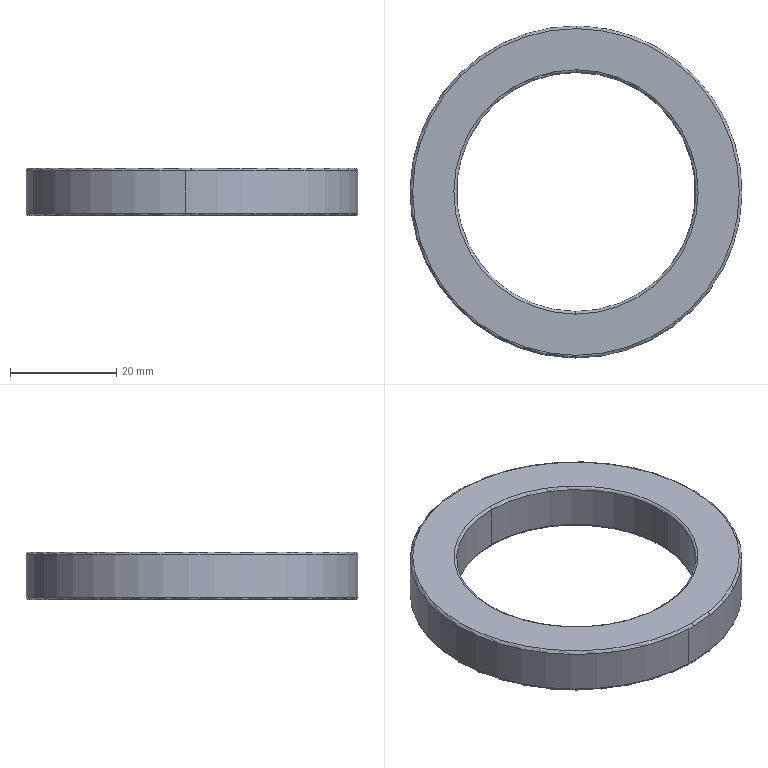Part | STEP file | 2026.6.15-Main Assembly图.sldasm-Part-147 | 1 solid | 14 faces | box 62.5 x 62.5 x 9 mm | volume 13262 mm3 | torus 8 | cylinder 4 | plane 2 | commonest cylinder face diameters 45 x2 62.5 x2
STEP:
#1=CARTESIAN_POINT('',(-1571.277,1393.006,3633.071));
#2=VERTEX_POINT('',#1);
#3=CARTESIAN_POINT('',(-1570.037,1455.482,3633.071));
#4=VERTEX_POINT('',#3);
#5=CARTESIAN_POINT('',(-1571.253,1424.256,3633.071));
#6=DIRECTION('',(0.,0.,1.));
#7=DIRECTION('',(0.0007664,1.,0.));
#8=AXIS2_PLACEMENT_3D('',#5,#6,#7);
#9=CIRCLE('',#8,31.25);
#10=EDGE_CURVE('',#2,#4,#9,.T.);
#11=ORIENTED_EDGE('',*,*,#10,.F.);
#12=CARTESIAN_POINT('',(-1571.277,1393.506,3632.571));
#13=VERTEX_POINT('',#12);
#14=CARTESIAN_POINT('',(-1571.277,1393.506,3633.071));
#15=DIRECTION('',(1.,-0.0007664,0.));
#16=DIRECTION('',(0.0007664,1.,0.));
#17=AXIS2_PLACEMENT_3D('',#14,#15,#16);
#18=CIRCLE('',#17,0.5);
#19=EDGE_CURVE('',#2,#13,#18,.T.);
#20=ORIENTED_EDGE('',*,*,#19,.T.);
#21=CARTESIAN_POINT('',(-1571.23,1455.006,3632.571));
#22=VERTEX_POINT('',#21);
#23=CARTESIAN_POINT('',(-1571.253,1424.256,3632.571));
#24=DIRECTION('',(0.,0.,-1.));
#25=DIRECTION('',(0.0007664,1.,0.));
#26=AXIS2_PLACEMENT_3D('',#23,#24,#25);
#27=CIRCLE('',#26,30.75);
#28=EDGE_CURVE('',#22,#13,#27,.T.);
#29=ORIENTED_EDGE('',*,*,#28,.F.);
#30=CARTESIAN_POINT('',(-1571.229,1455.506,3633.071));
#31=VERTEX_POINT('',#30);
#32=CARTESIAN_POINT('',(-1571.23,1455.006,3633.071));
#33=DIRECTION('',(-1.,0.0007664,0.));
#34=DIRECTION('',(-0.0007664,-1.,0.));
#35=AXIS2_PLACEMENT_3D('',#32,#33,#34);
#36=CIRCLE('',#35,0.5);
#37=EDGE_CURVE('',#31,#22,#36,.T.);
#38=ORIENTED_EDGE('',*,*,#37,.F.);
#39=CARTESIAN_POINT('',(-1571.253,1424.256,3633.071));
#40=DIRECTION('',(0.,0.,1.));
#41=DIRECTION('',(0.0007664,1.,0.));
#42=AXIS2_PLACEMENT_3D('',#39,#40,#41);
#43=CIRCLE('',#42,31.25);
#44=EDGE_CURVE('',#4,#31,#43,.T.);
#45=ORIENTED_EDGE('',*,*,#44,.F.);
#46=EDGE_LOOP('',(#11,#20,#29,#38,#45));
#47=FACE_OUTER_BOUND('',#46,.T.);
#48=CARTESIAN_POINT('',(-1571.253,1424.256,3633.071));
#49=DIRECTION('',(0.,0.,-1.));
#50=DIRECTION('',(0.0007664,1.,0.));
#51=AXIS2_PLACEMENT_3D('',#48,#49,#50);
#52=TOROIDAL_SURFACE('',#51,30.75,0.5);
#53=ADVANCED_FACE('',(#47),#52,.T.);
#54=CARTESIAN_POINT('',(-1571.229,1455.506,3641.071));
#55=VERTEX_POINT('',#54);
#56=CARTESIAN_POINT('',(-1570.037,1455.482,3641.071));
#57=VERTEX_POINT('',#56);
#58=CARTESIAN_POINT('',(-1571.253,1424.256,3641.071));
#59=DIRECTION('',(0.,0.,-1.));
#60=DIRECTION('',(-0.0007664,-1.,0.));
#61=AXIS2_PLACEMENT_3D('',#58,#59,#60);
#62=CIRCLE('',#61,31.25);
#63=EDGE_CURVE('',#55,#57,#62,.T.);
#64=ORIENTED_EDGE('',*,*,#63,.F.);
#65=CARTESIAN_POINT('',(-1571.23,1455.006,3641.571));
#66=VERTEX_POINT('',#65);
#67=CARTESIAN_POINT('',(-1571.23,1455.006,3641.071));
#68=DIRECTION('',(1.,-0.0007664,0.));
#69=DIRECTION('',(0.0007664,1.,0.));
#70=AXIS2_PLACEMENT_3D('',#67,#68,#69);
#71=CIRCLE('',#70,0.5);
#72=EDGE_CURVE('',#55,#66,#71,.T.);
#73=ORIENTED_EDGE('',*,*,#72,.T.);
#74=CARTESIAN_POINT('',(-1571.277,1393.506,3641.571));
#75=VERTEX_POINT('',#74);
#76=CARTESIAN_POINT('',(-1571.253,1424.256,3641.571));
#77=DIRECTION('',(0.,0.,1.));
#78=DIRECTION('',(-0.0007664,-1.,0.));
#79=AXIS2_PLACEMENT_3D('',#76,#77,#78);
#80=CIRCLE('',#79,30.75);
#81=EDGE_CURVE('',#75,#66,#80,.T.);
#82=ORIENTED_EDGE('',*,*,#81,.F.);
#83=CARTESIAN_POINT('',(-1571.277,1393.006,3641.071));
#84=VERTEX_POINT('',#83);
#85=CARTESIAN_POINT('',(-1571.277,1393.506,3641.071));
#86=DIRECTION('',(-1.,0.0007664,0.));
#87=DIRECTION('',(-0.0007664,-1.,0.));
#88=AXIS2_PLACEMENT_3D('',#85,#86,#87);
#89=CIRCLE('',#88,0.5);
#90=EDGE_CURVE('',#84,#75,#89,.T.);
#91=ORIENTED_EDGE('',*,*,#90,.F.);
#92=CARTESIAN_POINT('',(-1571.253,1424.256,3641.071));
#93=DIRECTION('',(0.,0.,-1.));
#94=DIRECTION('',(-0.0007664,-1.,0.));
#95=AXIS2_PLACEMENT_3D('',#92,#93,#94);
#96=CIRCLE('',#95,31.25);
#97=EDGE_CURVE('',#57,#84,#96,.T.);
#98=ORIENTED_EDGE('',*,*,#97,.F.);
#99=EDGE_LOOP('',(#64,#73,#82,#91,#98));
#100=FACE_OUTER_BOUND('',#99,.T.);
#101=CARTESIAN_POINT('',(-1571.253,1424.256,3641.071));
#102=DIRECTION('',(0.,0.,1.));
#103=DIRECTION('',(-0.0007664,-1.,0.));
#104=AXIS2_PLACEMENT_3D('',#101,#102,#103);
#105=TOROIDAL_SURFACE('',#104,30.75,0.5);
#106=ADVANCED_FACE('',(#100),#105,.T.);
#107=CARTESIAN_POINT('',(-1571.236,1447.256,3641.571));
#108=VERTEX_POINT('',#107);
#109=CARTESIAN_POINT('',(-1571.271,1401.256,3641.571));
#110=VERTEX_POINT('',#109);
#111=CARTESIAN_POINT('',(-1571.253,1424.256,3641.571));
#112=DIRECTION('',(0.,0.,-1.));
#113=DIRECTION('',(-0.0007664,-1.,0.));
#114=AXIS2_PLACEMENT_3D('',#111,#112,#113);
#115=CIRCLE('',#114,23.);
#116=EDGE_CURVE('',#108,#110,#115,.T.);
#117=ORIENTED_EDGE('',*,*,#116,.F.);
#118=CARTESIAN_POINT('',(-1571.236,1446.756,3641.071));
#119=VERTEX_POINT('',#118);
#120=CARTESIAN_POINT('',(-1571.236,1447.256,3641.071));
#121=DIRECTION('',(1.,-0.0007664,0.));
#122=DIRECTION('',(0.0007664,1.,0.));
#123=AXIS2_PLACEMENT_3D('',#120,#121,#122);
#124=CIRCLE('',#123,0.5);
#125=EDGE_CURVE('',#108,#119,#124,.T.);
#126=ORIENTED_EDGE('',*,*,#125,.T.);
#127=CARTESIAN_POINT('',(-1571.27,1401.756,3641.071));
#128=VERTEX_POINT('',#127);
#129=CARTESIAN_POINT('',(-1571.253,1424.256,3641.071));
#130=DIRECTION('',(0.,0.,1.));
#131=DIRECTION('',(-0.0007664,-1.,0.));
#132=AXIS2_PLACEMENT_3D('',#129,#130,#131);
#133=CIRCLE('',#132,22.5);
#134=EDGE_CURVE('',#128,#119,#133,.T.);
#135=ORIENTED_EDGE('',*,*,#134,.F.);
#136=CARTESIAN_POINT('',(-1571.271,1401.256,3641.071));
#137=DIRECTION('',(-1.,0.0007664,0.));
#138=DIRECTION('',(-0.0007664,-1.,0.));
#139=AXIS2_PLACEMENT_3D('',#136,#137,#138);
#140=CIRCLE('',#139,0.5);
#141=EDGE_CURVE('',#110,#128,#140,.T.);
#142=ORIENTED_EDGE('',*,*,#141,.F.);
#143=EDGE_LOOP('',(#117,#126,#135,#142));
#144=FACE_OUTER_BOUND('',#143,.T.);
#145=CARTESIAN_POINT('',(-1571.253,1424.256,3641.071));
#146=DIRECTION('',(0.,0.,1.));
#147=DIRECTION('',(-0.0007664,-1.,0.));
#148=AXIS2_PLACEMENT_3D('',#145,#146,#147);
#149=TOROIDAL_SURFACE('',#148,23.,0.5);
#150=ADVANCED_FACE('',(#144),#149,.T.);
#151=CARTESIAN_POINT('',(-1571.271,1401.256,3632.571));
#152=VERTEX_POINT('',#151);
#153=CARTESIAN_POINT('',(-1571.236,1447.256,3632.571));
#154=VERTEX_POINT('',#153);
#155=CARTESIAN_POINT('',(-1571.253,1424.256,3632.571));
#156=DIRECTION('',(0.,0.,1.));
#157=DIRECTION('',(0.0007664,1.,0.));
#158=AXIS2_PLACEMENT_3D('',#155,#156,#157);
#159=CIRCLE('',#158,23.);
#160=EDGE_CURVE('',#152,#154,#159,.T.);
#161=ORIENTED_EDGE('',*,*,#160,.F.);
#162=CARTESIAN_POINT('',(-1571.27,1401.756,3633.071));
#163=VERTEX_POINT('',#162);
#164=CARTESIAN_POINT('',(-1571.271,1401.256,3633.071));
#165=DIRECTION('',(1.,-0.0007664,0.));
#166=DIRECTION('',(0.0007664,1.,0.));
#167=AXIS2_PLACEMENT_3D('',#164,#165,#166);
#168=CIRCLE('',#167,0.5);
#169=EDGE_CURVE('',#152,#163,#168,.T.);
#170=ORIENTED_EDGE('',*,*,#169,.T.);
#171=CARTESIAN_POINT('',(-1571.236,1446.756,3633.071));
#172=VERTEX_POINT('',#171);
#173=CARTESIAN_POINT('',(-1571.253,1424.256,3633.071));
#174=DIRECTION('',(0.,0.,-1.));
#175=DIRECTION('',(0.0007664,1.,0.));
#176=AXIS2_PLACEMENT_3D('',#173,#174,#175);
#177=CIRCLE('',#176,22.5);
#178=EDGE_CURVE('',#172,#163,#177,.T.);
#179=ORIENTED_EDGE('',*,*,#178,.F.);
#180=CARTESIAN_POINT('',(-1571.236,1447.256,3633.071));
#181=DIRECTION('',(-1.,0.0007664,0.));
#182=DIRECTION('',(-0.0007664,-1.,0.));
#183=AXIS2_PLACEMENT_3D('',#180,#181,#182);
#184=CIRCLE('',#183,0.5);
#185=EDGE_CURVE('',#154,#172,#184,.T.);
#186=ORIENTED_EDGE('',*,*,#185,.F.);
#187=EDGE_LOOP('',(#161,#170,#179,#186));
#188=FACE_OUTER_BOUND('',#187,.T.);
#189=CARTESIAN_POINT('',(-1571.253,1424.256,3633.071));
#190=DIRECTION('',(0.,0.,-1.));
#191=DIRECTION('',(0.0007664,1.,0.));
#192=AXIS2_PLACEMENT_3D('',#189,#190,#191);
#193=TOROIDAL_SURFACE('',#192,23.,0.5);
#194=ADVANCED_FACE('',(#188),#193,.T.);
#195=CARTESIAN_POINT('',(-1571.253,1424.256,3633.071));
#196=DIRECTION('',(0.,0.,-1.));
#197=DIRECTION('',(0.0007664,1.,0.));
#198=AXIS2_PLACEMENT_3D('',#195,#196,#197);
#199=CIRCLE('',#198,22.5);
#200=EDGE_CURVE('',#163,#172,#199,.T.);
#201=ORIENTED_EDGE('',*,*,#200,.T.);
#202=CARTESIAN_POINT('',(-1571.236,1446.756,3632.571));
#203=DIRECTION('',(0.,0.,1.));
#204=VECTOR('',#203,1000.);
#205=LINE('',#202,#204);
#206=EDGE_CURVE('',#172,#119,#205,.T.);
#207=ORIENTED_EDGE('',*,*,#206,.T.);
#208=CARTESIAN_POINT('',(-1571.253,1424.256,3641.071));
#209=DIRECTION('',(0.,0.,1.));
#210=DIRECTION('',(-0.0007664,-1.,0.));
#211=AXIS2_PLACEMENT_3D('',#208,#209,#210);
#212=CIRCLE('',#211,22.5);
#213=EDGE_CURVE('',#119,#128,#212,.T.);
#214=ORIENTED_EDGE('',*,*,#213,.T.);
#215=CARTESIAN_POINT('',(-1571.27,1401.756,3632.571));
#216=DIRECTION('',(0.,0.,1.));
#217=VECTOR('',#216,1000.);
#218=LINE('',#215,#217);
#219=EDGE_CURVE('',#163,#128,#218,.T.);
#220=ORIENTED_EDGE('',*,*,#219,.F.);
#221=EDGE_LOOP('',(#201,#207,#214,#220));
#222=FACE_OUTER_BOUND('',#221,.T.);
#223=CARTESIAN_POINT('',(-1571.253,1424.256,3632.571));
#224=DIRECTION('',(0.,0.,1.));
#225=DIRECTION('',(-0.0007664,-1.,0.));
#226=AXIS2_PLACEMENT_3D('',#223,#224,#225);
#227=CYLINDRICAL_SURFACE('',#226,22.5);
#228=ADVANCED_FACE('',(#222),#227,.F.);
#229=ORIENTED_EDGE('',*,*,#97,.T.);
#230=CARTESIAN_POINT('',(-1572.469,1393.03,3641.071));
#231=VERTEX_POINT('',#230);
#232=CARTESIAN_POINT('',(-1571.253,1424.256,3641.071));
#233=DIRECTION('',(0.,0.,-1.));
#234=DIRECTION('',(-0.0007664,-1.,0.));
#235=AXIS2_PLACEMENT_3D('',#232,#233,#234);
#236=CIRCLE('',#235,31.25);
#237=EDGE_CURVE('',#84,#231,#236,.T.);
#238=ORIENTED_EDGE('',*,*,#237,.T.);
#239=CARTESIAN_POINT('',(-1572.469,1393.03,3633.071));
#240=VERTEX_POINT('',#239);
#241=CARTESIAN_POINT('',(-1572.469,1393.03,3641.571));
#242=DIRECTION('',(0.,0.,-1.));
#243=VECTOR('',#242,1000.);
#244=LINE('',#241,#243);
#245=EDGE_CURVE('',#231,#240,#244,.T.);
#246=ORIENTED_EDGE('',*,*,#245,.T.);
#247=CARTESIAN_POINT('',(-1571.253,1424.256,3633.071));
#248=DIRECTION('',(0.,0.,1.));
#249=DIRECTION('',(0.0007664,1.,0.));
#250=AXIS2_PLACEMENT_3D('',#247,#248,#249);
#251=CIRCLE('',#250,31.25);
#252=EDGE_CURVE('',#240,#2,#251,.T.);
#253=ORIENTED_EDGE('',*,*,#252,.T.);
#254=ORIENTED_EDGE('',*,*,#10,.T.);
#255=CARTESIAN_POINT('',(-1570.037,1455.482,3641.571));
#256=DIRECTION('',(0.,0.,-1.));
#257=VECTOR('',#256,1000.);
#258=LINE('',#255,#257);
#259=EDGE_CURVE('',#57,#4,#258,.T.);
#260=ORIENTED_EDGE('',*,*,#259,.F.);
#261=EDGE_LOOP('',(#229,#238,#246,#253,#254,#260));
#262=FACE_OUTER_BOUND('',#261,.T.);
#263=CARTESIAN_POINT('',(-1571.253,1424.256,3641.571));
#264=DIRECTION('',(0.,0.,-1.));
#265=DIRECTION('',(0.03892,0.9992,0.));
#266=AXIS2_PLACEMENT_3D('',#263,#264,#265);
#267=CYLINDRICAL_SURFACE('',#266,31.25);
#268=ADVANCED_FACE('',(#262),#267,.T.);
#269=CARTESIAN_POINT('',(-1571.253,1424.256,3632.571));
#270=DIRECTION('',(0.,0.,1.));
#271=DIRECTION('',(0.0007664,1.,0.));
#272=AXIS2_PLACEMENT_3D('',#269,#270,#271);
#273=CIRCLE('',#272,23.);
#274=EDGE_CURVE('',#154,#152,#273,.T.);
#275=ORIENTED_EDGE('',*,*,#274,.T.);
#276=ORIENTED_EDGE('',*,*,#160,.T.);
#277=EDGE_LOOP('',(#275,#276));
#278=FACE_BOUND('',#277,.T.);
#279=ORIENTED_EDGE('',*,*,#28,.T.);
#280=CARTESIAN_POINT('',(-1571.253,1424.256,3632.571));
#281=DIRECTION('',(0.,0.,-1.));
#282=DIRECTION('',(0.0007664,1.,0.));
#283=AXIS2_PLACEMENT_3D('',#280,#281,#282);
#284=CIRCLE('',#283,30.75);
#285=EDGE_CURVE('',#13,#22,#284,.T.);
#286=ORIENTED_EDGE('',*,*,#285,.T.);
#287=EDGE_LOOP('',(#279,#286));
#288=FACE_OUTER_BOUND('',#287,.T.);
#289=CARTESIAN_POINT('',(-1571.253,1424.256,3632.571));
#290=DIRECTION('',(0.,0.,-1.));
#291=DIRECTION('',(0.0007664,1.,0.));
#292=AXIS2_PLACEMENT_3D('',#289,#290,#291);
#293=PLANE('',#292);
#294=ADVANCED_FACE('',(#278,#288),#293,.T.);
#295=CARTESIAN_POINT('',(-1571.253,1424.256,3641.571));
#296=DIRECTION('',(0.,0.,-1.));
#297=DIRECTION('',(-0.0007664,-1.,0.));
#298=AXIS2_PLACEMENT_3D('',#295,#296,#297);
#299=CIRCLE('',#298,23.);
#300=EDGE_CURVE('',#110,#108,#299,.T.);
#301=ORIENTED_EDGE('',*,*,#300,.T.);
#302=ORIENTED_EDGE('',*,*,#116,.T.);
#303=EDGE_LOOP('',(#301,#302));
#304=FACE_BOUND('',#303,.T.);
#305=ORIENTED_EDGE('',*,*,#81,.T.);
#306=CARTESIAN_POINT('',(-1571.253,1424.256,3641.571));
#307=DIRECTION('',(0.,0.,1.));
#308=DIRECTION('',(-0.0007664,-1.,0.));
#309=AXIS2_PLACEMENT_3D('',#306,#307,#308);
#310=CIRCLE('',#309,30.75);
#311=EDGE_CURVE('',#66,#75,#310,.T.);
#312=ORIENTED_EDGE('',*,*,#311,.T.);
#313=EDGE_LOOP('',(#305,#312));
#314=FACE_OUTER_BOUND('',#313,.T.);
#315=CARTESIAN_POINT('',(-1571.253,1424.256,3641.571));
#316=DIRECTION('',(0.,0.,1.));
#317=DIRECTION('',(-0.0007664,-1.,0.));
#318=AXIS2_PLACEMENT_3D('',#315,#316,#317);
#319=PLANE('',#318);
#320=ADVANCED_FACE('',(#304,#314),#319,.T.);
#321=ORIENTED_EDGE('',*,*,#245,.F.);
#322=CARTESIAN_POINT('',(-1571.253,1424.256,3641.071));
#323=DIRECTION('',(0.,0.,-1.));
#324=DIRECTION('',(-0.0007664,-1.,0.));
#325=AXIS2_PLACEMENT_3D('',#322,#323,#324);
#326=CIRCLE('',#325,31.25);
#327=EDGE_CURVE('',#231,#55,#326,.T.);
#328=ORIENTED_EDGE('',*,*,#327,.T.);
#329=ORIENTED_EDGE('',*,*,#63,.T.);
#330=ORIENTED_EDGE('',*,*,#259,.T.);
#331=ORIENTED_EDGE('',*,*,#44,.T.);
#332=CARTESIAN_POINT('',(-1571.253,1424.256,3633.071));
#333=DIRECTION('',(0.,0.,1.));
#334=DIRECTION('',(0.0007664,1.,0.));
#335=AXIS2_PLACEMENT_3D('',#332,#333,#334);
#336=CIRCLE('',#335,31.25);
#337=EDGE_CURVE('',#31,#240,#336,.T.);
#338=ORIENTED_EDGE('',*,*,#337,.T.);
#339=EDGE_LOOP('',(#321,#328,#329,#330,#331,#338));
#340=FACE_OUTER_BOUND('',#339,.T.);
#341=CARTESIAN_POINT('',(-1571.253,1424.256,3641.571));
#342=DIRECTION('',(0.,0.,-1.));
#343=DIRECTION('',(0.03892,0.9992,0.));
#344=AXIS2_PLACEMENT_3D('',#341,#342,#343);
#345=CYLINDRICAL_SURFACE('',#344,31.25);
#346=ADVANCED_FACE('',(#340),#345,.T.);
#347=ORIENTED_EDGE('',*,*,#206,.F.);
#348=ORIENTED_EDGE('',*,*,#178,.T.);
#349=ORIENTED_EDGE('',*,*,#219,.T.);
#350=ORIENTED_EDGE('',*,*,#134,.T.);
#351=EDGE_LOOP('',(#347,#348,#349,#350));
#352=FACE_OUTER_BOUND('',#351,.T.);
#353=CARTESIAN_POINT('',(-1571.253,1424.256,3632.571));
#354=DIRECTION('',(0.,0.,1.));
#355=DIRECTION('',(-0.0007664,-1.,0.));
#356=AXIS2_PLACEMENT_3D('',#353,#354,#355);
#357=CYLINDRICAL_SURFACE('',#356,22.5);
#358=ADVANCED_FACE('',(#352),#357,.F.);
#359=ORIENTED_EDGE('',*,*,#169,.F.);
#360=ORIENTED_EDGE('',*,*,#274,.F.);
#361=ORIENTED_EDGE('',*,*,#185,.T.);
#362=ORIENTED_EDGE('',*,*,#200,.F.);
#363=EDGE_LOOP('',(#359,#360,#361,#362));
#364=FACE_OUTER_BOUND('',#363,.T.);
#365=CARTESIAN_POINT('',(-1571.253,1424.256,3633.071));
#366=DIRECTION('',(0.,0.,-1.));
#367=DIRECTION('',(0.0007664,1.,0.));
#368=AXIS2_PLACEMENT_3D('',#365,#366,#367);
#369=TOROIDAL_SURFACE('',#368,23.,0.5);
#370=ADVANCED_FACE('',(#364),#369,.T.);
#371=ORIENTED_EDGE('',*,*,#125,.F.);
#372=ORIENTED_EDGE('',*,*,#300,.F.);
#373=ORIENTED_EDGE('',*,*,#141,.T.);
#374=ORIENTED_EDGE('',*,*,#213,.F.);
#375=EDGE_LOOP('',(#371,#372,#373,#374));
#376=FACE_OUTER_BOUND('',#375,.T.);
#377=CARTESIAN_POINT('',(-1571.253,1424.256,3641.071));
#378=DIRECTION('',(0.,0.,1.));
#379=DIRECTION('',(-0.0007664,-1.,0.));
#380=AXIS2_PLACEMENT_3D('',#377,#378,#379);
#381=TOROIDAL_SURFACE('',#380,23.,0.5);
#382=ADVANCED_FACE('',(#376),#381,.T.);
#383=ORIENTED_EDGE('',*,*,#72,.F.);
#384=ORIENTED_EDGE('',*,*,#327,.F.);
#385=ORIENTED_EDGE('',*,*,#237,.F.);
#386=ORIENTED_EDGE('',*,*,#90,.T.);
#387=ORIENTED_EDGE('',*,*,#311,.F.);
#388=EDGE_LOOP('',(#383,#384,#385,#386,#387));
#389=FACE_OUTER_BOUND('',#388,.T.);
#390=CARTESIAN_POINT('',(-1571.253,1424.256,3641.071));
#391=DIRECTION('',(0.,0.,1.));
#392=DIRECTION('',(-0.0007664,-1.,0.));
#393=AXIS2_PLACEMENT_3D('',#390,#391,#392);
#394=TOROIDAL_SURFACE('',#393,30.75,0.5);
#395=ADVANCED_FACE('',(#389),#394,.T.);
#396=ORIENTED_EDGE('',*,*,#19,.F.);
#397=ORIENTED_EDGE('',*,*,#252,.F.);
#398=ORIENTED_EDGE('',*,*,#337,.F.);
#399=ORIENTED_EDGE('',*,*,#37,.T.);
#400=ORIENTED_EDGE('',*,*,#285,.F.);
#401=EDGE_LOOP('',(#396,#397,#398,#399,#400));
#402=FACE_OUTER_BOUND('',#401,.T.);
#403=CARTESIAN_POINT('',(-1571.253,1424.256,3633.071));
#404=DIRECTION('',(0.,0.,-1.));
#405=DIRECTION('',(0.0007664,1.,0.));
#406=AXIS2_PLACEMENT_3D('',#403,#404,#405);
#407=TOROIDAL_SURFACE('',#406,30.75,0.5);
#408=ADVANCED_FACE('',(#402),#407,.T.);
#409=CLOSED_SHELL('',(#53,#106,#150,#194,#228,#268,#294,#320,#346,#358,#370,#382,#395,#408));
#410=MANIFOLD_SOLID_BREP('',#409);
#411=CARTESIAN_POINT('',(0.,0.,0.));
#412=DIRECTION('',(0.,0.,1.));
#413=DIRECTION('',(1.,0.,0.));
#414=AXIS2_PLACEMENT_3D('',#411,#412,#413);
#415=(LENGTH_UNIT()NAMED_UNIT(*)SI_UNIT(.MILLI.,.METRE.));
#416=UNCERTAINTY_MEASURE_WITH_UNIT(LENGTH_MEASURE(0.00001),#415,'','');
#417=(NAMED_UNIT(*)PLANE_ANGLE_UNIT()SI_UNIT($,.RADIAN.));
#418=(NAMED_UNIT(*)SI_UNIT($,.STERADIAN.)SOLID_ANGLE_UNIT());
#419=(GEOMETRIC_REPRESENTATION_CONTEXT(3)GLOBAL_UNCERTAINTY_ASSIGNED_CONTEXT((#416))GLOBAL_UNIT_ASSIGNED_CONTEXT((#415,#417,#418))REPRESENTATION_CONTEXT('',''));
#420=ADVANCED_BREP_SHAPE_REPRESENTATION('',(#410,#414),#419);